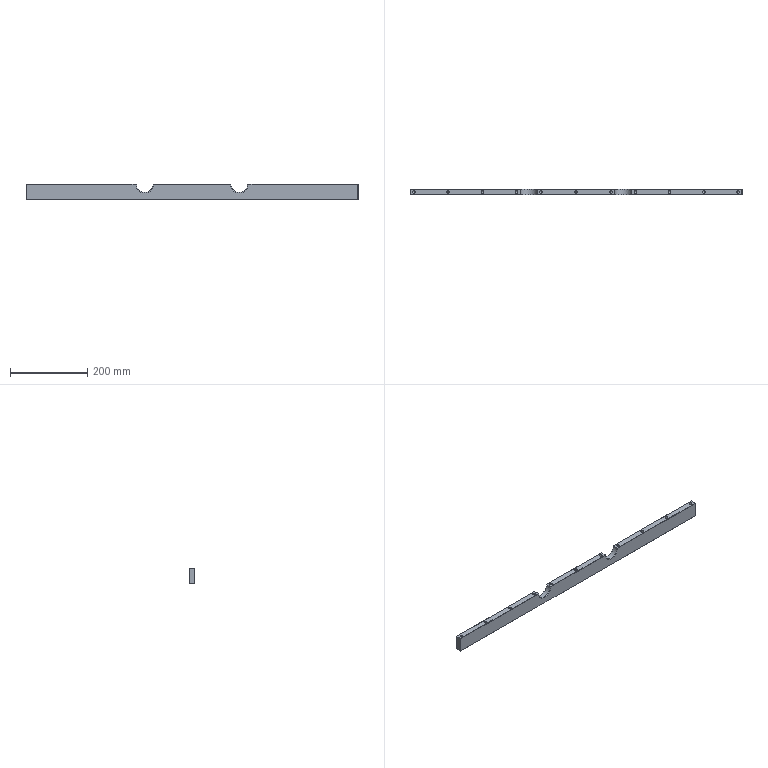Part | SolidWorks | features Chamfer 3, Extrusion 1, HoleWzd 1, ICE 1 | 1 solid | 88 faces | box 860 x 15 x 40 mm | volume 485456 mm3 | plane 36 | cone 28 | cylinder 24 | commonest cylinder face diameters 6.8 x22 43 x2